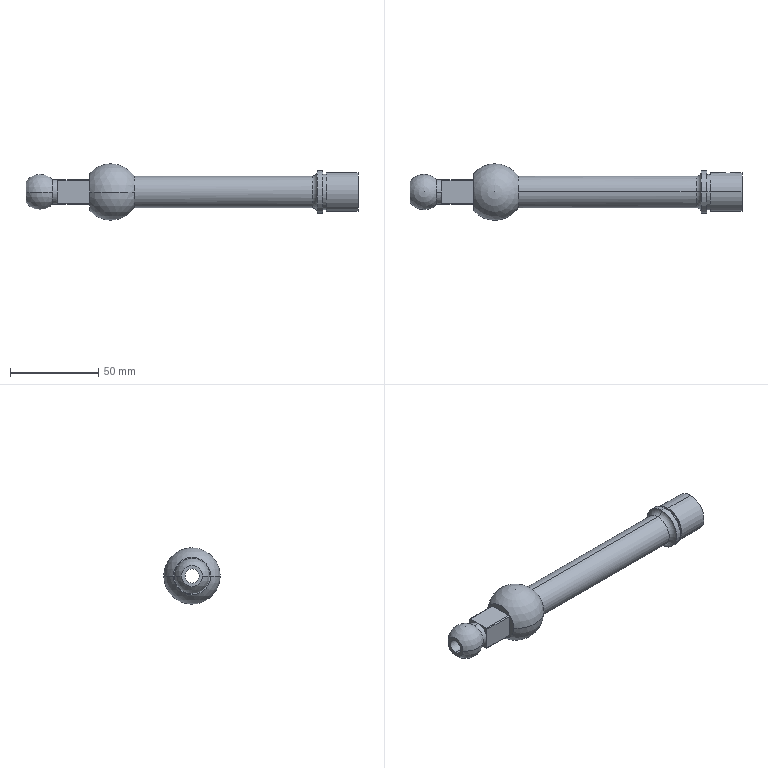Part | SolidWorks | features ICE 2, Revolution 1 | 1 solid | 42 faces | box 188 x 32 x 32 mm | volume 46322 mm3 | cylinder 20 | plane 14 | sphere 4 | torus 2 | cone 2 | commonest cylinder face diameters 19 x4 5 x2 8 x2 14 x2 17.3 x2 18 x2
STEP:
#1=CARTESIAN_POINT('',(246.379,32.914,-2.5));
#2=VERTEX_POINT('',#1);
#3=CARTESIAN_POINT('',(246.379,32.914,2.5));
#4=VERTEX_POINT('',#3);
#5=CARTESIAN_POINT('',(246.379,32.914,-2.5));
#6=CARTESIAN_POINT('',(246.214,32.914,-2.5));
#7=CARTESIAN_POINT('',(246.051,32.918,-2.484));
#8=CARTESIAN_POINT('',(245.73,32.932,-2.42));
#9=CARTESIAN_POINT('',(245.571,32.943,-2.371));
#10=CARTESIAN_POINT('',(245.269,32.97,-2.246));
#11=CARTESIAN_POINT('',(245.125,32.986,-2.169));
#12=CARTESIAN_POINT('',(244.854,33.021,-1.988));
#13=CARTESIAN_POINT('',(244.726,33.04,-1.882));
#14=CARTESIAN_POINT('',(244.381,33.096,-1.538));
#15=CARTESIAN_POINT('',(244.195,33.133,-1.259));
#16=CARTESIAN_POINT('',(244.008,33.173,-0.8084));
#17=CARTESIAN_POINT('',(243.96,33.184,-0.6503));
#18=CARTESIAN_POINT('',(243.895,33.198,-0.3273));
#19=CARTESIAN_POINT('',(243.879,33.202,-0.1647));
#20=CARTESIAN_POINT('',(243.879,33.202,0.1627));
#21=CARTESIAN_POINT('',(243.896,33.198,0.329));
#22=CARTESIAN_POINT('',(243.96,33.184,0.65));
#23=CARTESIAN_POINT('',(244.007,33.173,0.8062));
#24=CARTESIAN_POINT('',(244.196,33.133,1.261));
#25=CARTESIAN_POINT('',(244.38,33.096,1.536));
#26=CARTESIAN_POINT('',(244.728,33.04,1.884));
#27=CARTESIAN_POINT('',(244.854,33.021,1.987));
#28=CARTESIAN_POINT('',(245.124,32.986,2.168));
#29=CARTESIAN_POINT('',(245.27,32.97,2.247));
#30=CARTESIAN_POINT('',(245.572,32.943,2.372));
#31=CARTESIAN_POINT('',(245.728,32.932,2.419));
#32=CARTESIAN_POINT('',(246.05,32.918,2.484));
#33=CARTESIAN_POINT('',(246.216,32.914,2.5));
#34=CARTESIAN_POINT('',(246.379,32.914,2.5));
#35=B_SPLINE_CURVE_WITH_KNOTS('',3,(#5,#6,#7,#8,#9,#10,#11,#12,#13,#14,#15,#16,#17,#18,#19,#20,#21,#22,#23,#24,#25,#26,#27,#28,#29,#30,#31,#32,#33,#34),.UNSPECIFIED.,.F.,.F.,(4,2,2,2,2,2,2,2,2,2,2,2,2,2,4),(0.,0.0004901,0.0009802,0.00147,0.00196,0.002941,0.003431,0.003921,0.004411,0.004901,0.005881,0.006371,0.006862,0.007352,0.007842),.UNSPECIFIED.);
#36=EDGE_CURVE('',#2,#4,#35,.T.);
#37=ORIENTED_EDGE('',*,*,#36,.T.);
#38=CARTESIAN_POINT('',(246.379,30.482,2.5));
#39=VERTEX_POINT('',#38);
#40=CARTESIAN_POINT('',(246.379,39.202,2.5));
#41=DIRECTION('',(0.,-1.,0.));
#42=VECTOR('',#41,1000.);
#43=LINE('',#40,#42);
#44=EDGE_CURVE('',#4,#39,#43,.T.);
#45=ORIENTED_EDGE('',*,*,#44,.T.);
#46=CARTESIAN_POINT('',(246.379,30.482,-2.5));
#47=VERTEX_POINT('',#46);
#48=CARTESIAN_POINT('',(246.379,30.482,2.5));
#49=CARTESIAN_POINT('',(246.052,30.482,2.5));
#50=CARTESIAN_POINT('',(245.721,30.503,2.434));
#51=CARTESIAN_POINT('',(245.27,30.555,2.246));
#52=CARTESIAN_POINT('',(245.123,30.576,2.168));
#53=CARTESIAN_POINT('',(244.853,30.621,1.986));
#54=CARTESIAN_POINT('',(244.727,30.645,1.884));
#55=CARTESIAN_POINT('',(244.497,30.693,1.653));
#56=CARTESIAN_POINT('',(244.392,30.717,1.526));
#57=CARTESIAN_POINT('',(244.212,30.761,1.256));
#58=CARTESIAN_POINT('',(244.135,30.781,1.113));
#59=CARTESIAN_POINT('',(244.008,30.815,0.8077));
#60=CARTESIAN_POINT('',(243.96,30.829,0.6513));
#61=CARTESIAN_POINT('',(243.896,30.847,0.331));
#62=CARTESIAN_POINT('',(243.879,30.852,0.1651));
#63=CARTESIAN_POINT('',(243.879,30.852,-0.1645));
#64=CARTESIAN_POINT('',(243.895,30.847,-0.3273));
#65=CARTESIAN_POINT('',(243.959,30.829,-0.6493));
#66=CARTESIAN_POINT('',(244.008,30.815,-0.8088));
#67=CARTESIAN_POINT('',(244.196,30.765,-1.261));
#68=CARTESIAN_POINT('',(244.382,30.717,-1.538));
#69=CARTESIAN_POINT('',(244.726,30.645,-1.882));
#70=CARTESIAN_POINT('',(244.853,30.621,-1.987));
#71=CARTESIAN_POINT('',(245.124,30.576,-2.168));
#72=CARTESIAN_POINT('',(245.267,30.555,-2.245));
#73=CARTESIAN_POINT('',(245.569,30.521,-2.37));
#74=CARTESIAN_POINT('',(245.728,30.506,-2.419));
#75=CARTESIAN_POINT('',(246.05,30.487,-2.484));
#76=CARTESIAN_POINT('',(246.213,30.482,-2.5));
#77=CARTESIAN_POINT('',(246.379,30.482,-2.5));
#78=B_SPLINE_CURVE_WITH_KNOTS('',3,(#48,#49,#50,#51,#52,#53,#54,#55,#56,#57,#58,#59,#60,#61,#62,#63,#64,#65,#66,#67,#68,#69,#70,#71,#72,#73,#74,#75,#76,#77),.UNSPECIFIED.,.F.,.F.,(4,2,2,2,2,2,2,2,2,2,2,2,2,2,4),(0.007858,0.00884,0.009331,0.009822,0.01031,0.0108,0.0113,0.01179,0.01228,0.01277,0.01375,0.01424,0.01473,0.01522,0.01571),.UNSPECIFIED.);
#79=EDGE_CURVE('',#39,#47,#78,.T.);
#80=ORIENTED_EDGE('',*,*,#79,.T.);
#81=CARTESIAN_POINT('',(246.379,39.202,-2.5));
#82=DIRECTION('',(0.,-1.,0.));
#83=VECTOR('',#82,1000.);
#84=LINE('',#81,#83);
#85=EDGE_CURVE('',#2,#47,#84,.T.);
#86=ORIENTED_EDGE('',*,*,#85,.F.);
#87=EDGE_LOOP('',(#37,#45,#80,#86));
#88=FACE_OUTER_BOUND('',#87,.T.);
#89=CARTESIAN_POINT('',(246.379,39.202,0.));
#90=DIRECTION('',(0.,-1.,0.));
#91=DIRECTION('',(0.,0.,-1.));
#92=AXIS2_PLACEMENT_3D('',#89,#90,#91);
#93=CYLINDRICAL_SURFACE('',#92,2.5);
#94=ADVANCED_FACE('',(#88),#93,.F.);
#95=CARTESIAN_POINT('',(228.379,22.202,9.));
#96=VERTEX_POINT('',#95);
#97=CARTESIAN_POINT('',(228.379,22.202,-9.));
#98=VERTEX_POINT('',#97);
#99=CARTESIAN_POINT('',(228.379,22.202,0.));
#100=DIRECTION('',(-1.,0.,0.));
#101=DIRECTION('',(0.,0.,1.));
#102=AXIS2_PLACEMENT_3D('',#99,#100,#101);
#103=CIRCLE('',#102,9.);
#104=EDGE_CURVE('',#96,#98,#103,.T.);
#105=ORIENTED_EDGE('',*,*,#104,.T.);
#106=CARTESIAN_POINT('',(127.608,22.202,-9.));
#107=VERTEX_POINT('',#106);
#108=CARTESIAN_POINT('',(62.379,22.202,-9.));
#109=DIRECTION('',(-1.,0.,0.));
#110=VECTOR('',#109,1000.);
#111=LINE('',#108,#110);
#112=EDGE_CURVE('',#98,#107,#111,.T.);
#113=ORIENTED_EDGE('',*,*,#112,.T.);
#114=CARTESIAN_POINT('',(127.608,31.202,0.));
#115=VERTEX_POINT('',#114);
#116=CARTESIAN_POINT('',(127.608,22.202,0.));
#117=DIRECTION('',(-1.,0.,0.));
#118=DIRECTION('',(0.,0.,1.));
#119=AXIS2_PLACEMENT_3D('',#116,#117,#118);
#120=CIRCLE('',#119,9.);
#121=EDGE_CURVE('',#115,#107,#120,.T.);
#122=ORIENTED_EDGE('',*,*,#121,.F.);
#123=CARTESIAN_POINT('',(127.608,22.202,9.));
#124=VERTEX_POINT('',#123);
#125=CARTESIAN_POINT('',(127.608,22.202,0.));
#126=DIRECTION('',(-1.,0.,0.));
#127=DIRECTION('',(0.,0.,1.));
#128=AXIS2_PLACEMENT_3D('',#125,#126,#127);
#129=CIRCLE('',#128,9.);
#130=EDGE_CURVE('',#124,#115,#129,.T.);
#131=ORIENTED_EDGE('',*,*,#130,.F.);
#132=CARTESIAN_POINT('',(62.379,22.202,9.));
#133=DIRECTION('',(-1.,0.,0.));
#134=VECTOR('',#133,1000.);
#135=LINE('',#132,#134);
#136=EDGE_CURVE('',#96,#124,#135,.T.);
#137=ORIENTED_EDGE('',*,*,#136,.F.);
#138=EDGE_LOOP('',(#105,#113,#122,#131,#137));
#139=FACE_OUTER_BOUND('',#138,.T.);
#140=CARTESIAN_POINT('',(62.379,22.202,0.));
#141=DIRECTION('',(-1.,0.,0.));
#142=DIRECTION('',(0.,0.,1.));
#143=AXIS2_PLACEMENT_3D('',#140,#141,#142);
#144=CYLINDRICAL_SURFACE('',#143,9.);
#145=ADVANCED_FACE('',(#139),#144,.T.);
#146=CARTESIAN_POINT('',(228.379,22.202,0.));
#147=DIRECTION('',(-1.,0.,0.));
#148=DIRECTION('',(0.,0.,1.));
#149=AXIS2_PLACEMENT_3D('',#146,#147,#148);
#150=CIRCLE('',#149,9.);
#151=EDGE_CURVE('',#98,#96,#150,.T.);
#152=ORIENTED_EDGE('',*,*,#151,.F.);
#153=CARTESIAN_POINT('',(231.379,22.202,-12.));
#154=VERTEX_POINT('',#153);
#155=CARTESIAN_POINT('',(228.379,22.202,-12.));
#156=DIRECTION('',(0.,1.,0.));
#157=DIRECTION('',(0.,0.,1.));
#158=AXIS2_PLACEMENT_3D('',#155,#156,#157);
#159=CIRCLE('',#158,3.);
#160=EDGE_CURVE('',#98,#154,#159,.T.);
#161=ORIENTED_EDGE('',*,*,#160,.T.);
#162=CARTESIAN_POINT('',(231.379,22.202,12.));
#163=VERTEX_POINT('',#162);
#164=CARTESIAN_POINT('',(231.379,22.202,0.));
#165=DIRECTION('',(-1.,0.,0.));
#166=DIRECTION('',(0.,0.,1.));
#167=AXIS2_PLACEMENT_3D('',#164,#165,#166);
#168=CIRCLE('',#167,12.);
#169=EDGE_CURVE('',#154,#163,#168,.T.);
#170=ORIENTED_EDGE('',*,*,#169,.T.);
#171=CARTESIAN_POINT('',(228.379,22.202,12.));
#172=DIRECTION('',(0.,-1.,0.));
#173=DIRECTION('',(0.,0.,-1.));
#174=AXIS2_PLACEMENT_3D('',#171,#172,#173);
#175=CIRCLE('',#174,3.);
#176=EDGE_CURVE('',#96,#163,#175,.T.);
#177=ORIENTED_EDGE('',*,*,#176,.F.);
#178=EDGE_LOOP('',(#152,#161,#170,#177));
#179=FACE_OUTER_BOUND('',#178,.T.);
#180=CARTESIAN_POINT('',(228.379,22.202,0.));
#181=DIRECTION('',(-1.,0.,0.));
#182=DIRECTION('',(0.,0.,1.));
#183=AXIS2_PLACEMENT_3D('',#180,#181,#182);
#184=TOROIDAL_SURFACE('',#183,12.,3.);
#185=ADVANCED_FACE('',(#179),#184,.F.);
#186=CARTESIAN_POINT('',(234.379,22.202,12.));
#187=VERTEX_POINT('',#186);
#188=CARTESIAN_POINT('',(234.379,22.202,-12.));
#189=VERTEX_POINT('',#188);
#190=CARTESIAN_POINT('',(234.379,22.202,0.));
#191=DIRECTION('',(-1.,0.,0.));
#192=DIRECTION('',(0.,0.,1.));
#193=AXIS2_PLACEMENT_3D('',#190,#191,#192);
#194=CIRCLE('',#193,12.);
#195=EDGE_CURVE('',#187,#189,#194,.T.);
#196=ORIENTED_EDGE('',*,*,#195,.T.);
#197=CARTESIAN_POINT('',(62.379,22.202,-12.));
#198=DIRECTION('',(-1.,0.,0.));
#199=VECTOR('',#198,1000.);
#200=LINE('',#197,#199);
#201=EDGE_CURVE('',#189,#154,#200,.T.);
#202=ORIENTED_EDGE('',*,*,#201,.T.);
#203=CARTESIAN_POINT('',(231.379,22.202,0.));
#204=DIRECTION('',(-1.,0.,0.));
#205=DIRECTION('',(0.,0.,1.));
#206=AXIS2_PLACEMENT_3D('',#203,#204,#205);
#207=CIRCLE('',#206,12.);
#208=EDGE_CURVE('',#163,#154,#207,.T.);
#209=ORIENTED_EDGE('',*,*,#208,.F.);
#210=CARTESIAN_POINT('',(62.379,22.202,12.));
#211=DIRECTION('',(-1.,0.,0.));
#212=VECTOR('',#211,1000.);
#213=LINE('',#210,#212);
#214=EDGE_CURVE('',#187,#163,#213,.T.);
#215=ORIENTED_EDGE('',*,*,#214,.F.);
#216=EDGE_LOOP('',(#196,#202,#209,#215));
#217=FACE_OUTER_BOUND('',#216,.T.);
#218=CARTESIAN_POINT('',(62.379,22.202,0.));
#219=DIRECTION('',(-1.,0.,0.));
#220=DIRECTION('',(0.,0.,1.));
#221=AXIS2_PLACEMENT_3D('',#218,#219,#220);
#222=CYLINDRICAL_SURFACE('',#221,12.);
#223=ADVANCED_FACE('',(#217),#222,.T.);
#224=CARTESIAN_POINT('',(236.379,22.202,10.));
#225=VERTEX_POINT('',#224);
#226=CARTESIAN_POINT('',(236.379,22.202,-10.));
#227=VERTEX_POINT('',#226);
#228=CARTESIAN_POINT('',(236.379,22.202,0.));
#229=DIRECTION('',(-1.,0.,0.));
#230=DIRECTION('',(0.,0.,1.));
#231=AXIS2_PLACEMENT_3D('',#228,#229,#230);
#232=CIRCLE('',#231,10.);
#233=EDGE_CURVE('',#225,#227,#232,.T.);
#234=ORIENTED_EDGE('',*,*,#233,.T.);
#235=CARTESIAN_POINT('',(234.379,22.202,-10.));
#236=VERTEX_POINT('',#235);
#237=CARTESIAN_POINT('',(62.379,22.202,-10.));
#238=DIRECTION('',(-1.,0.,0.));
#239=VECTOR('',#238,1000.);
#240=LINE('',#237,#239);
#241=EDGE_CURVE('',#227,#236,#240,.T.);
#242=ORIENTED_EDGE('',*,*,#241,.T.);
#243=CARTESIAN_POINT('',(234.379,22.202,10.));
#244=VERTEX_POINT('',#243);
#245=CARTESIAN_POINT('',(234.379,22.202,0.));
#246=DIRECTION('',(-1.,0.,0.));
#247=DIRECTION('',(0.,0.,1.));
#248=AXIS2_PLACEMENT_3D('',#245,#246,#247);
#249=CIRCLE('',#248,10.);
#250=EDGE_CURVE('',#244,#236,#249,.T.);
#251=ORIENTED_EDGE('',*,*,#250,.F.);
#252=CARTESIAN_POINT('',(62.379,22.202,10.));
#253=DIRECTION('',(-1.,0.,0.));
#254=VECTOR('',#253,1000.);
#255=LINE('',#252,#254);
#256=EDGE_CURVE('',#225,#244,#255,.T.);
#257=ORIENTED_EDGE('',*,*,#256,.F.);
#258=EDGE_LOOP('',(#234,#242,#251,#257));
#259=FACE_OUTER_BOUND('',#258,.T.);
#260=CARTESIAN_POINT('',(62.379,22.202,0.));
#261=DIRECTION('',(-1.,0.,0.));
#262=DIRECTION('',(0.,0.,1.));
#263=AXIS2_PLACEMENT_3D('',#260,#261,#262);
#264=CYLINDRICAL_SURFACE('',#263,10.);
#265=ADVANCED_FACE('',(#259),#264,.T.);
#266=CARTESIAN_POINT('',(234.379,22.202,-4.));
#267=VERTEX_POINT('',#266);
#268=CARTESIAN_POINT('',(234.379,22.202,4.));
#269=VERTEX_POINT('',#268);
#270=CARTESIAN_POINT('',(234.379,22.202,0.));
#271=DIRECTION('',(-1.,0.,0.));
#272=DIRECTION('',(0.,0.,1.));
#273=AXIS2_PLACEMENT_3D('',#270,#271,#272);
#274=CIRCLE('',#273,4.);
#275=EDGE_CURVE('',#267,#269,#274,.T.);
#276=ORIENTED_EDGE('',*,*,#275,.T.);
#277=CARTESIAN_POINT('',(237.379,22.202,8.65));
#278=VERTEX_POINT('',#277);
#279=CARTESIAN_POINT('',(234.379,22.202,4.));
#280=DIRECTION('',(0.5421,0.,0.8403));
#281=VECTOR('',#280,1000.);
#282=LINE('',#279,#281);
#283=EDGE_CURVE('',#269,#278,#282,.T.);
#284=ORIENTED_EDGE('',*,*,#283,.T.);
#285=CARTESIAN_POINT('',(237.379,22.202,-8.65));
#286=VERTEX_POINT('',#285);
#287=CARTESIAN_POINT('',(237.379,22.202,0.));
#288=DIRECTION('',(-1.,0.,0.));
#289=DIRECTION('',(0.,0.,1.));
#290=AXIS2_PLACEMENT_3D('',#287,#288,#289);
#291=CIRCLE('',#290,8.65);
#292=EDGE_CURVE('',#286,#278,#291,.T.);
#293=ORIENTED_EDGE('',*,*,#292,.F.);
#294=CARTESIAN_POINT('',(234.379,22.202,-4.));
#295=DIRECTION('',(0.5421,0.,-0.8403));
#296=VECTOR('',#295,1000.);
#297=LINE('',#294,#296);
#298=EDGE_CURVE('',#267,#286,#297,.T.);
#299=ORIENTED_EDGE('',*,*,#298,.F.);
#300=EDGE_LOOP('',(#276,#284,#293,#299));
#301=FACE_OUTER_BOUND('',#300,.T.);
#302=CARTESIAN_POINT('',(234.379,22.202,0.));
#303=DIRECTION('',(1.,0.,0.));
#304=DIRECTION('',(0.,0.,-1.));
#305=AXIS2_PLACEMENT_3D('',#302,#303,#304);
#306=CONICAL_SURFACE('',#305,4.,0.9978);
#307=ADVANCED_FACE('',(#301),#306,.F.);
#308=ORIENTED_EDGE('',*,*,#275,.F.);
#309=CARTESIAN_POINT('',(66.379,22.202,-4.));
#310=VERTEX_POINT('',#309);
#311=CARTESIAN_POINT('',(62.379,22.202,-4.));
#312=DIRECTION('',(-1.,0.,0.));
#313=VECTOR('',#312,1000.);
#314=LINE('',#311,#313);
#315=EDGE_CURVE('',#267,#310,#314,.T.);
#316=ORIENTED_EDGE('',*,*,#315,.T.);
#317=CARTESIAN_POINT('',(66.379,22.202,4.));
#318=VERTEX_POINT('',#317);
#319=CARTESIAN_POINT('',(66.379,22.202,0.));
#320=DIRECTION('',(-1.,0.,0.));
#321=DIRECTION('',(0.,0.,1.));
#322=AXIS2_PLACEMENT_3D('',#319,#320,#321);
#323=CIRCLE('',#322,4.);
#324=EDGE_CURVE('',#310,#318,#323,.T.);
#325=ORIENTED_EDGE('',*,*,#324,.T.);
#326=CARTESIAN_POINT('',(62.379,22.202,4.));
#327=DIRECTION('',(-1.,0.,0.));
#328=VECTOR('',#327,1000.);
#329=LINE('',#326,#328);
#330=EDGE_CURVE('',#269,#318,#329,.T.);
#331=ORIENTED_EDGE('',*,*,#330,.F.);
#332=EDGE_LOOP('',(#308,#316,#325,#331));
#333=FACE_OUTER_BOUND('',#332,.T.);
#334=CARTESIAN_POINT('',(62.379,22.202,0.));
#335=DIRECTION('',(-1.,0.,0.));
#336=DIRECTION('',(0.,0.,1.));
#337=AXIS2_PLACEMENT_3D('',#334,#335,#336);
#338=CYLINDRICAL_SURFACE('',#337,4.);
#339=ADVANCED_FACE('',(#333),#338,.F.);
#340=CARTESIAN_POINT('',(81.379,29.343,0.));
#341=VERTEX_POINT('',#340);
#342=CARTESIAN_POINT('',(81.379,15.06,0.));
#343=VERTEX_POINT('',#342);
#344=CARTESIAN_POINT('',(81.379,22.202,0.));
#345=DIRECTION('',(-1.,0.,0.));
#346=DIRECTION('',(0.,0.,1.));
#347=AXIS2_PLACEMENT_3D('',#344,#345,#346);
#348=CIRCLE('',#347,7.141);
#349=EDGE_CURVE('',#341,#343,#348,.T.);
#350=ORIENTED_EDGE('',*,*,#349,.T.);
#351=CARTESIAN_POINT('',(66.379,16.202,0.));
#352=VERTEX_POINT('',#351);
#353=CARTESIAN_POINT('',(74.379,22.202,0.));
#354=DIRECTION('',(0.,0.,-1.));
#355=DIRECTION('',(0.,1.,0.));
#356=AXIS2_PLACEMENT_3D('',#353,#354,#355);
#357=CIRCLE('',#356,10.);
#358=EDGE_CURVE('',#343,#352,#357,.T.);
#359=ORIENTED_EDGE('',*,*,#358,.T.);
#360=CARTESIAN_POINT('',(66.379,28.202,0.));
#361=VERTEX_POINT('',#360);
#362=CARTESIAN_POINT('',(66.379,22.202,0.));
#363=DIRECTION('',(-1.,0.,0.));
#364=DIRECTION('',(0.,0.,1.));
#365=AXIS2_PLACEMENT_3D('',#362,#363,#364);
#366=CIRCLE('',#365,6.);
#367=EDGE_CURVE('',#361,#352,#366,.T.);
#368=ORIENTED_EDGE('',*,*,#367,.F.);
#369=CARTESIAN_POINT('',(74.379,22.202,0.));
#370=DIRECTION('',(0.,0.,1.));
#371=DIRECTION('',(1.,0.,0.));
#372=AXIS2_PLACEMENT_3D('',#369,#370,#371);
#373=CIRCLE('',#372,10.);
#374=EDGE_CURVE('',#341,#361,#373,.T.);
#375=ORIENTED_EDGE('',*,*,#374,.F.);
#376=EDGE_LOOP('',(#350,#359,#368,#375));
#377=FACE_OUTER_BOUND('',#376,.T.);
#378=CARTESIAN_POINT('',(74.379,22.202,0.));
#379=DIRECTION('',(0.,0.,-1.));
#380=DIRECTION('',(0.,1.,0.));
#381=AXIS2_PLACEMENT_3D('',#378,#379,#380);
#382=SPHERICAL_SURFACE('',#381,10.);
#383=ADVANCED_FACE('',(#377),#382,.T.);
#384=CARTESIAN_POINT('',(84.379,29.202,0.));
#385=VERTEX_POINT('',#384);
#386=CARTESIAN_POINT('',(84.379,22.202,-7.));
#387=VERTEX_POINT('',#386);
#388=CARTESIAN_POINT('',(84.379,22.202,0.));
#389=DIRECTION('',(-1.,0.,0.));
#390=DIRECTION('',(0.,0.,1.));
#391=AXIS2_PLACEMENT_3D('',#388,#389,#390);
#392=CIRCLE('',#391,7.);
#393=EDGE_CURVE('',#385,#387,#392,.T.);
#394=ORIENTED_EDGE('',*,*,#393,.T.);
#395=CARTESIAN_POINT('',(81.379,22.202,-7.));
#396=VERTEX_POINT('',#395);
#397=CARTESIAN_POINT('',(62.379,22.202,-7.));
#398=DIRECTION('',(-1.,0.,0.));
#399=VECTOR('',#398,1000.);
#400=LINE('',#397,#399);
#401=EDGE_CURVE('',#387,#396,#400,.T.);
#402=ORIENTED_EDGE('',*,*,#401,.T.);
#403=CARTESIAN_POINT('',(81.379,22.202,7.));
#404=VERTEX_POINT('',#403);
#405=CARTESIAN_POINT('',(81.379,22.202,0.));
#406=DIRECTION('',(-1.,0.,0.));
#407=DIRECTION('',(0.,0.,1.));
#408=AXIS2_PLACEMENT_3D('',#405,#406,#407);
#409=CIRCLE('',#408,7.);
#410=EDGE_CURVE('',#404,#396,#409,.T.);
#411=ORIENTED_EDGE('',*,*,#410,.F.);
#412=CARTESIAN_POINT('',(84.379,22.202,7.));
#413=VERTEX_POINT('',#412);
#414=CARTESIAN_POINT('',(62.379,22.202,7.));
#415=DIRECTION('',(-1.,0.,0.));
#416=VECTOR('',#415,1000.);
#417=LINE('',#414,#416);
#418=EDGE_CURVE('',#413,#404,#417,.T.);
#419=ORIENTED_EDGE('',*,*,#418,.F.);
#420=CARTESIAN_POINT('',(84.379,22.202,0.));
#421=DIRECTION('',(-1.,0.,0.));
#422=DIRECTION('',(0.,0.,1.));
#423=AXIS2_PLACEMENT_3D('',#420,#421,#422);
#424=CIRCLE('',#423,7.);
#425=EDGE_CURVE('',#413,#385,#424,.T.);
#426=ORIENTED_EDGE('',*,*,#425,.T.);
#427=EDGE_LOOP('',(#394,#402,#411,#419,#426));
#428=FACE_OUTER_BOUND('',#427,.T.);
#429=CARTESIAN_POINT('',(62.379,22.202,0.));
#430=DIRECTION('',(-1.,0.,0.));
#431=DIRECTION('',(0.,0.,1.));
#432=AXIS2_PLACEMENT_3D('',#429,#430,#431);
#433=CYLINDRICAL_SURFACE('',#432,7.);
#434=ADVANCED_FACE('',(#428),#433,.T.);
#435=ORIENTED_EDGE('',*,*,#121,.T.);
#436=CARTESIAN_POINT('',(127.608,13.202,0.));
#437=VERTEX_POINT('',#436);
#438=CARTESIAN_POINT('',(127.608,22.202,0.));
#439=DIRECTION('',(-1.,0.,0.));
#440=DIRECTION('',(0.,0.,1.));
#441=AXIS2_PLACEMENT_3D('',#438,#439,#440);
#442=CIRCLE('',#441,9.);
#443=EDGE_CURVE('',#107,#437,#442,.T.);
#444=ORIENTED_EDGE('',*,*,#443,.T.);
#445=CARTESIAN_POINT('',(102.379,11.619,0.));
#446=VERTEX_POINT('',#445);
#447=CARTESIAN_POINT('',(114.379,22.202,0.));
#448=DIRECTION('',(0.,0.,-1.));
#449=DIRECTION('',(0.,1.,0.));
#450=AXIS2_PLACEMENT_3D('',#447,#448,#449);
#451=CIRCLE('',#450,16.);
#452=EDGE_CURVE('',#437,#446,#451,.T.);
#453=ORIENTED_EDGE('',*,*,#452,.T.);
#454=CARTESIAN_POINT('',(102.379,32.785,0.));
#455=VERTEX_POINT('',#454);
#456=CARTESIAN_POINT('',(102.379,22.202,0.));
#457=DIRECTION('',(-1.,0.,0.));
#458=DIRECTION('',(0.,0.,1.));
#459=AXIS2_PLACEMENT_3D('',#456,#457,#458);
#460=CIRCLE('',#459,10.583);
#461=EDGE_CURVE('',#455,#446,#460,.T.);
#462=ORIENTED_EDGE('',*,*,#461,.F.);
#463=CARTESIAN_POINT('',(114.379,22.202,0.));
#464=DIRECTION('',(0.,0.,1.));
#465=DIRECTION('',(1.,0.,0.));
#466=AXIS2_PLACEMENT_3D('',#463,#464,#465);
#467=CIRCLE('',#466,16.);
#468=EDGE_CURVE('',#115,#455,#467,.T.);
#469=ORIENTED_EDGE('',*,*,#468,.F.);
#470=EDGE_LOOP('',(#435,#444,#453,#462,#469));
#471=FACE_OUTER_BOUND('',#470,.T.);
#472=CARTESIAN_POINT('',(114.379,22.202,0.));
#473=DIRECTION('',(0.,0.,-1.));
#474=DIRECTION('',(0.,1.,0.));
#475=AXIS2_PLACEMENT_3D('',#472,#473,#474);
#476=SPHERICAL_SURFACE('',#475,16.);
#477=ADVANCED_FACE('',(#471),#476,.T.);
#478=ORIENTED_EDGE('',*,*,#36,.F.);
#479=CARTESIAN_POINT('',(246.379,32.914,2.5));
#480=CARTESIAN_POINT('',(246.706,32.914,2.5));
#481=CARTESIAN_POINT('',(247.036,32.93,2.434));
#482=CARTESIAN_POINT('',(247.488,32.97,2.247));
#483=CARTESIAN_POINT('',(247.634,32.986,2.169));
#484=CARTESIAN_POINT('',(247.905,33.021,1.987));
#485=CARTESIAN_POINT('',(248.031,33.04,1.884));
#486=CARTESIAN_POINT('',(248.261,33.077,1.654));
#487=CARTESIAN_POINT('',(248.367,33.096,1.525));
#488=CARTESIAN_POINT('',(248.547,33.131,1.255));
#489=CARTESIAN_POINT('',(248.624,33.146,1.112));
#490=CARTESIAN_POINT('',(248.814,33.186,0.6562));
#491=CARTESIAN_POINT('',(248.879,33.202,0.3309));
#492=CARTESIAN_POINT('',(248.879,33.202,-0.164));
#493=CARTESIAN_POINT('',(248.863,33.198,-0.3266));
#494=CARTESIAN_POINT('',(248.8,33.184,-0.6474));
#495=CARTESIAN_POINT('',(248.751,33.173,-0.8069));
#496=CARTESIAN_POINT('',(248.626,33.147,-1.109));
#497=CARTESIAN_POINT('',(248.549,33.131,-1.252));
#498=CARTESIAN_POINT('',(248.367,33.096,-1.525));
#499=CARTESIAN_POINT('',(248.263,33.077,-1.652));
#500=CARTESIAN_POINT('',(247.919,33.021,-1.996));
#501=CARTESIAN_POINT('',(247.641,32.984,-2.183));
#502=CARTESIAN_POINT('',(247.19,32.943,-2.371));
#503=CARTESIAN_POINT('',(247.031,32.932,-2.419));
#504=CARTESIAN_POINT('',(246.708,32.918,-2.484));
#505=CARTESIAN_POINT('',(246.545,32.914,-2.5));
#506=CARTESIAN_POINT('',(246.379,32.914,-2.5));
#507=B_SPLINE_CURVE_WITH_KNOTS('',3,(#479,#480,#481,#482,#483,#484,#485,#486,#487,#488,#489,#490,#491,#492,#493,#494,#495,#496,#497,#498,#499,#500,#501,#502,#503,#504,#505,#506),.UNSPECIFIED.,.F.,.F.,(4,2,2,2,2,2,2,2,2,2,2,2,2,4),(0.007842,0.008822,0.009312,0.009802,0.01029,0.01078,0.01176,0.01225,0.01274,0.01323,0.01372,0.0147,0.01519,0.01568),.UNSPECIFIED.);
#508=EDGE_CURVE('',#4,#2,#507,.T.);
#509=ORIENTED_EDGE('',*,*,#508,.F.);
#510=EDGE_LOOP('',(#478,#509));
#511=FACE_BOUND('',#510,.T.);
#512=CARTESIAN_POINT('',(254.379,22.202,11.));
#513=VERTEX_POINT('',#512);
#514=CARTESIAN_POINT('',(254.379,22.202,-11.));
#515=VERTEX_POINT('',#514);
#516=CARTESIAN_POINT('',(254.379,22.202,0.));
#517=DIRECTION('',(-1.,0.,0.));
#518=DIRECTION('',(0.,0.,1.));
#519=AXIS2_PLACEMENT_3D('',#516,#517,#518);
#520=CIRCLE('',#519,11.);
#521=EDGE_CURVE('',#513,#515,#520,.T.);
#522=ORIENTED_EDGE('',*,*,#521,.T.);
#523=CARTESIAN_POINT('',(236.379,22.202,-11.));
#524=VERTEX_POINT('',#523);
#525=CARTESIAN_POINT('',(62.379,22.202,-11.));
#526=DIRECTION('',(-1.,0.,0.));
#527=VECTOR('',#526,1000.);
#528=LINE('',#525,#527);
#529=EDGE_CURVE('',#515,#524,#528,.T.);
#530=ORIENTED_EDGE('',*,*,#529,.T.);
#531=CARTESIAN_POINT('',(236.379,22.202,11.));
#532=VERTEX_POINT('',#531);
#533=CARTESIAN_POINT('',(236.379,22.202,0.));
#534=DIRECTION('',(-1.,0.,0.));
#535=DIRECTION('',(0.,0.,1.));
#536=AXIS2_PLACEMENT_3D('',#533,#534,#535);
#537=CIRCLE('',#536,11.);
#538=EDGE_CURVE('',#532,#524,#537,.T.);
#539=ORIENTED_EDGE('',*,*,#538,.F.);
#540=CARTESIAN_POINT('',(62.379,22.202,11.));
#541=DIRECTION('',(-1.,0.,0.));
#542=VECTOR('',#541,1000.);
#543=LINE('',#540,#542);
#544=EDGE_CURVE('',#513,#532,#543,.T.);
#545=ORIENTED_EDGE('',*,*,#544,.F.);
#546=EDGE_LOOP('',(#522,#530,#539,#545));
#547=FACE_OUTER_BOUND('',#546,.T.);
#548=CARTESIAN_POINT('',(62.379,22.202,0.));
#549=DIRECTION('',(-1.,0.,0.));
#550=DIRECTION('',(0.,0.,1.));
#551=AXIS2_PLACEMENT_3D('',#548,#549,#550);
#552=CYLINDRICAL_SURFACE('',#551,11.);
#553=ADVANCED_FACE('',(#511,#547),#552,.T.);
#554=CARTESIAN_POINT('',(254.379,22.202,-8.65));
#555=VERTEX_POINT('',#554);
#556=CARTESIAN_POINT('',(254.379,22.202,8.65));
#557=VERTEX_POINT('',#556);
#558=CARTESIAN_POINT('',(254.379,22.202,0.));
#559=DIRECTION('',(-1.,0.,0.));
#560=DIRECTION('',(0.,0.,1.));
#561=AXIS2_PLACEMENT_3D('',#558,#559,#560);
#562=CIRCLE('',#561,8.65);
#563=EDGE_CURVE('',#555,#557,#562,.T.);
#564=ORIENTED_EDGE('',*,*,#563,.F.);
#565=CARTESIAN_POINT('',(62.379,22.202,-8.65));
#566=DIRECTION('',(-1.,0.,0.));
#567=VECTOR('',#566,1000.);
#568=LINE('',#565,#567);
#569=EDGE_CURVE('',#555,#286,#568,.T.);
#570=ORIENTED_EDGE('',*,*,#569,.T.);
#571=ORIENTED_EDGE('',*,*,#292,.T.);
#572=CARTESIAN_POINT('',(62.379,22.202,8.65));
#573=DIRECTION('',(-1.,0.,0.));
#574=VECTOR('',#573,1000.);
#575=LINE('',#572,#574);
#576=EDGE_CURVE('',#557,#278,#575,.T.);
#577=ORIENTED_EDGE('',*,*,#576,.F.);
#578=EDGE_LOOP('',(#564,#570,#571,#577));
#579=FACE_OUTER_BOUND('',#578,.T.);
#580=CARTESIAN_POINT('',(62.379,22.202,0.));
#581=DIRECTION('',(-1.,0.,0.));
#582=DIRECTION('',(0.,0.,1.));
#583=AXIS2_PLACEMENT_3D('',#580,#581,#582);
#584=CYLINDRICAL_SURFACE('',#583,8.65);
#585=ADVANCED_FACE('',(#579),#584,.F.);
#586=ORIENTED_EDGE('',*,*,#569,.F.);
#587=CARTESIAN_POINT('',(254.379,22.202,0.));
#588=DIRECTION('',(-1.,0.,0.));
#589=DIRECTION('',(0.,0.,1.));
#590=AXIS2_PLACEMENT_3D('',#587,#588,#589);
#591=CIRCLE('',#590,8.65);
#592=EDGE_CURVE('',#557,#555,#591,.T.);
#593=ORIENTED_EDGE('',*,*,#592,.F.);
#594=ORIENTED_EDGE('',*,*,#576,.T.);
#595=CARTESIAN_POINT('',(237.379,22.202,0.));
#596=DIRECTION('',(-1.,0.,0.));
#597=DIRECTION('',(0.,0.,1.));
#598=AXIS2_PLACEMENT_3D('',#595,#596,#597);
#599=CIRCLE('',#598,8.65);
#600=EDGE_CURVE('',#278,#286,#599,.T.);
#601=ORIENTED_EDGE('',*,*,#600,.T.);
#602=EDGE_LOOP('',(#586,#593,#594,#601));
#603=FACE_OUTER_BOUND('',#602,.T.);
#604=CARTESIAN_POINT('',(246.379,30.482,-2.5));
#605=CARTESIAN_POINT('',(246.545,30.482,-2.5));
#606=CARTESIAN_POINT('',(246.709,30.487,-2.484));
#607=CARTESIAN_POINT('',(247.029,30.506,-2.42));
#608=CARTESIAN_POINT('',(247.189,30.521,-2.371));
#609=CARTESIAN_POINT('',(247.491,30.555,-2.245));
#610=CARTESIAN_POINT('',(247.634,30.576,-2.168));
#611=CARTESIAN_POINT('',(247.905,30.621,-1.987));
#612=CARTESIAN_POINT('',(248.033,30.645,-1.882));
#613=CARTESIAN_POINT('',(248.377,30.717,-1.538));
#614=CARTESIAN_POINT('',(248.563,30.765,-1.261));
#615=CARTESIAN_POINT('',(248.75,30.815,-0.8097));
#616=CARTESIAN_POINT('',(248.799,30.829,-0.6512));
#617=CARTESIAN_POINT('',(248.863,30.847,-0.328));
#618=CARTESIAN_POINT('',(248.879,30.852,-0.1651));
#619=CARTESIAN_POINT('',(248.879,30.852,0.163));
#620=CARTESIAN_POINT('',(248.863,30.847,0.3297));
#621=CARTESIAN_POINT('',(248.799,30.829,0.6511));
#622=CARTESIAN_POINT('',(248.751,30.815,0.8074));
#623=CARTESIAN_POINT('',(248.562,30.764,1.263));
#624=CARTESIAN_POINT('',(248.377,30.717,1.538));
#625=CARTESIAN_POINT('',(248.031,30.645,1.884));
#626=CARTESIAN_POINT('',(247.905,30.621,1.987));
#627=CARTESIAN_POINT('',(247.635,30.576,2.168));
#628=CARTESIAN_POINT('',(247.489,30.555,2.246));
#629=CARTESIAN_POINT('',(247.187,30.52,2.371));
#630=CARTESIAN_POINT('',(247.032,30.507,2.419));
#631=CARTESIAN_POINT('',(246.709,30.487,2.484));
#632=CARTESIAN_POINT('',(246.543,30.482,2.5));
#633=CARTESIAN_POINT('',(246.379,30.482,2.5));
#634=B_SPLINE_CURVE_WITH_KNOTS('',3,(#604,#605,#606,#607,#608,#609,#610,#611,#612,#613,#614,#615,#616,#617,#618,#619,#620,#621,#622,#623,#624,#625,#626,#627,#628,#629,#630,#631,#632,#633),.UNSPECIFIED.,.F.,.F.,(4,2,2,2,2,2,2,2,2,2,2,2,2,2,4),(0.,0.0004911,0.0009823,0.001473,0.001965,0.002947,0.003438,0.003929,0.00442,0.004911,0.005894,0.006385,0.006876,0.007367,0.007858),.UNSPECIFIED.);
#635=EDGE_CURVE('',#47,#39,#634,.T.);
#636=ORIENTED_EDGE('',*,*,#635,.F.);
#637=ORIENTED_EDGE('',*,*,#79,.F.);
#638=EDGE_LOOP('',(#636,#637));
#639=FACE_BOUND('',#638,.T.);
#640=CARTESIAN_POINT('',(62.379,22.202,0.));
#641=DIRECTION('',(-1.,0.,0.));
#642=DIRECTION('',(0.,0.,1.));
#643=AXIS2_PLACEMENT_3D('',#640,#641,#642);
#644=CYLINDRICAL_SURFACE('',#643,8.65);
#645=ADVANCED_FACE('',(#603,#639),#644,.F.);
#646=ORIENTED_EDGE('',*,*,#529,.F.);
#647=CARTESIAN_POINT('',(254.379,22.202,0.));
#648=DIRECTION('',(-1.,0.,0.));
#649=DIRECTION('',(0.,0.,1.));
#650=AXIS2_PLACEMENT_3D('',#647,#648,#649);
#651=CIRCLE('',#650,11.);
#652=EDGE_CURVE('',#515,#513,#651,.T.);
#653=ORIENTED_EDGE('',*,*,#652,.T.);
#654=ORIENTED_EDGE('',*,*,#544,.T.);
#655=CARTESIAN_POINT('',(236.379,22.202,0.));
#656=DIRECTION('',(-1.,0.,0.));
#657=DIRECTION('',(0.,0.,1.));
#658=AXIS2_PLACEMENT_3D('',#655,#656,#657);
#659=CIRCLE('',#658,11.);
#660=EDGE_CURVE('',#524,#532,#659,.T.);
#661=ORIENTED_EDGE('',*,*,#660,.F.);
#662=EDGE_LOOP('',(#646,#653,#654,#661));
#663=FACE_OUTER_BOUND('',#662,.T.);
#664=CARTESIAN_POINT('',(62.379,22.202,0.));
#665=DIRECTION('',(-1.,0.,0.));
#666=DIRECTION('',(0.,0.,1.));
#667=AXIS2_PLACEMENT_3D('',#664,#665,#666);
#668=CYLINDRICAL_SURFACE('',#667,11.);
#669=ADVANCED_FACE('',(#663),#668,.T.);
#670=CARTESIAN_POINT('',(102.379,28.624,7.));
#671=VERTEX_POINT('',#670);
#672=CARTESIAN_POINT('',(84.379,28.624,7.));
#673=VERTEX_POINT('',#672);
#674=CARTESIAN_POINT('',(62.379,28.624,7.));
#675=DIRECTION('',(-1.,0.,0.));
#676=VECTOR('',#675,1000.);
#677=LINE('',#674,#676);
#678=EDGE_CURVE('',#671,#673,#677,.T.);
#679=ORIENTED_EDGE('',*,*,#678,.F.);
#680=CARTESIAN_POINT('',(102.379,29.202,6.423));
#681=VERTEX_POINT('',#680);
#682=CARTESIAN_POINT('',(102.379,22.202,0.));
#683=DIRECTION('',(-1.,0.,0.));
#684=DIRECTION('',(0.,0.,1.));
#685=AXIS2_PLACEMENT_3D('',#682,#683,#684);
#686=CIRCLE('',#685,9.5);
#687=EDGE_CURVE('',#671,#681,#686,.T.);
#688=ORIENTED_EDGE('',*,*,#687,.T.);
#689=CARTESIAN_POINT('',(84.379,29.202,6.423));
#690=VERTEX_POINT('',#689);
#691=CARTESIAN_POINT('',(62.379,29.202,6.423));
#692=DIRECTION('',(1.,0.,0.));
#693=VECTOR('',#692,1000.);
#694=LINE('',#691,#693);
#695=EDGE_CURVE('',#690,#681,#694,.T.);
#696=ORIENTED_EDGE('',*,*,#695,.F.);
#697=CARTESIAN_POINT('',(84.379,22.202,0.));
#698=DIRECTION('',(-1.,0.,0.));
#699=DIRECTION('',(0.,0.,1.));
#700=AXIS2_PLACEMENT_3D('',#697,#698,#699);
#701=CIRCLE('',#700,9.5);
#702=EDGE_CURVE('',#673,#690,#701,.T.);
#703=ORIENTED_EDGE('',*,*,#702,.F.);
#704=EDGE_LOOP('',(#679,#688,#696,#703));
#705=FACE_OUTER_BOUND('',#704,.T.);
#706=CARTESIAN_POINT('',(62.379,22.202,0.));
#707=DIRECTION('',(-1.,0.,0.));
#708=DIRECTION('',(0.,0.,1.));
#709=AXIS2_PLACEMENT_3D('',#706,#707,#708);
#710=CYLINDRICAL_SURFACE('',#709,9.5);
#711=ADVANCED_FACE('',(#705),#710,.T.);
#712=CARTESIAN_POINT('',(84.379,15.779,7.));
#713=VERTEX_POINT('',#712);
#714=CARTESIAN_POINT('',(102.379,15.779,7.));
#715=VERTEX_POINT('',#714);
#716=CARTESIAN_POINT('',(62.379,15.779,7.));
#717=DIRECTION('',(1.,0.,0.));
#718=VECTOR('',#717,1000.);
#719=LINE('',#716,#718);
#720=EDGE_CURVE('',#713,#715,#719,.T.);
#721=ORIENTED_EDGE('',*,*,#720,.F.);
#722=CARTESIAN_POINT('',(84.379,15.202,6.423));
#723=VERTEX_POINT('',#722);
#724=CARTESIAN_POINT('',(84.379,22.202,0.));
#725=DIRECTION('',(-1.,0.,0.));
#726=DIRECTION('',(0.,0.,1.));
#727=AXIS2_PLACEMENT_3D('',#724,#725,#726);
#728=CIRCLE('',#727,9.5);
#729=EDGE_CURVE('',#723,#713,#728,.T.);
#730=ORIENTED_EDGE('',*,*,#729,.F.);
#731=CARTESIAN_POINT('',(102.379,15.202,6.423));
#732=VERTEX_POINT('',#731);
#733=CARTESIAN_POINT('',(62.379,15.202,6.423));
#734=DIRECTION('',(-1.,0.,0.));
#735=VECTOR('',#734,1000.);
#736=LINE('',#733,#735);
#737=EDGE_CURVE('',#732,#723,#736,.T.);
#738=ORIENTED_EDGE('',*,*,#737,.F.);
#739=CARTESIAN_POINT('',(102.379,22.202,0.));
#740=DIRECTION('',(-1.,0.,0.));
#741=DIRECTION('',(0.,0.,1.));
#742=AXIS2_PLACEMENT_3D('',#739,#740,#741);
#743=CIRCLE('',#742,9.5);
#744=EDGE_CURVE('',#732,#715,#743,.T.);
#745=ORIENTED_EDGE('',*,*,#744,.T.);
#746=EDGE_LOOP('',(#721,#730,#738,#745));
#747=FACE_OUTER_BOUND('',#746,.T.);
#748=CARTESIAN_POINT('',(62.379,22.202,0.));
#749=DIRECTION('',(-1.,0.,0.));
#750=DIRECTION('',(0.,0.,1.));
#751=AXIS2_PLACEMENT_3D('',#748,#749,#750);
#752=CYLINDRICAL_SURFACE('',#751,9.5);
#753=ADVANCED_FACE('',(#747),#752,.T.);
#754=CARTESIAN_POINT('',(84.379,15.202,-6.423));
#755=VERTEX_POINT('',#754);
#756=CARTESIAN_POINT('',(102.379,15.202,-6.423));
#757=VERTEX_POINT('',#756);
#758=CARTESIAN_POINT('',(62.379,15.202,-6.423));
#759=DIRECTION('',(1.,0.,0.));
#760=VECTOR('',#759,1000.);
#761=LINE('',#758,#760);
#762=EDGE_CURVE('',#755,#757,#761,.T.);
#763=ORIENTED_EDGE('',*,*,#762,.F.);
#764=CARTESIAN_POINT('',(84.379,15.779,-7.));
#765=VERTEX_POINT('',#764);
#766=CARTESIAN_POINT('',(84.379,22.202,0.));
#767=DIRECTION('',(-1.,0.,0.));
#768=DIRECTION('',(0.,0.,1.));
#769=AXIS2_PLACEMENT_3D('',#766,#767,#768);
#770=CIRCLE('',#769,9.5);
#771=EDGE_CURVE('',#765,#755,#770,.T.);
#772=ORIENTED_EDGE('',*,*,#771,.F.);
#773=CARTESIAN_POINT('',(102.379,15.779,-7.));
#774=VERTEX_POINT('',#773);
#775=CARTESIAN_POINT('',(62.379,15.779,-7.));
#776=DIRECTION('',(-1.,0.,0.));
#777=VECTOR('',#776,1000.);
#778=LINE('',#775,#777);
#779=EDGE_CURVE('',#774,#765,#778,.T.);
#780=ORIENTED_EDGE('',*,*,#779,.F.);
#781=CARTESIAN_POINT('',(102.379,22.202,0.));
#782=DIRECTION('',(-1.,0.,0.));
#783=DIRECTION('',(0.,0.,1.));
#784=AXIS2_PLACEMENT_3D('',#781,#782,#783);
#785=CIRCLE('',#784,9.5);
#786=EDGE_CURVE('',#774,#757,#785,.T.);
#787=ORIENTED_EDGE('',*,*,#786,.T.);
#788=EDGE_LOOP('',(#763,#772,#780,#787));
#789=FACE_OUTER_BOUND('',#788,.T.);
#790=CARTESIAN_POINT('',(62.379,22.202,0.));
#791=DIRECTION('',(-1.,0.,0.));
#792=DIRECTION('',(0.,0.,1.));
#793=AXIS2_PLACEMENT_3D('',#790,#791,#792);
#794=CYLINDRICAL_SURFACE('',#793,9.5);
#795=ADVANCED_FACE('',(#789),#794,.T.);
#796=CARTESIAN_POINT('',(84.379,28.624,-7.));
#797=VERTEX_POINT('',#796);
#798=CARTESIAN_POINT('',(102.379,28.624,-7.));
#799=VERTEX_POINT('',#798);
#800=CARTESIAN_POINT('',(62.379,28.624,-7.));
#801=DIRECTION('',(1.,0.,0.));
#802=VECTOR('',#801,1000.);
#803=LINE('',#800,#802);
#804=EDGE_CURVE('',#797,#799,#803,.T.);
#805=ORIENTED_EDGE('',*,*,#804,.F.);
#806=CARTESIAN_POINT('',(84.379,29.202,-6.423));
#807=VERTEX_POINT('',#806);
#808=CARTESIAN_POINT('',(84.379,22.202,0.));
#809=DIRECTION('',(-1.,0.,0.));
#810=DIRECTION('',(0.,0.,1.));
#811=AXIS2_PLACEMENT_3D('',#808,#809,#810);
#812=CIRCLE('',#811,9.5);
#813=EDGE_CURVE('',#807,#797,#812,.T.);
#814=ORIENTED_EDGE('',*,*,#813,.F.);
#815=CARTESIAN_POINT('',(102.379,29.202,-6.423));
#816=VERTEX_POINT('',#815);
#817=CARTESIAN_POINT('',(62.379,29.202,-6.423));
#818=DIRECTION('',(-1.,0.,0.));
#819=VECTOR('',#818,1000.);
#820=LINE('',#817,#819);
#821=EDGE_CURVE('',#816,#807,#820,.T.);
#822=ORIENTED_EDGE('',*,*,#821,.F.);
#823=CARTESIAN_POINT('',(102.379,22.202,0.));
#824=DIRECTION('',(-1.,0.,0.));
#825=DIRECTION('',(0.,0.,1.));
#826=AXIS2_PLACEMENT_3D('',#823,#824,#825);
#827=CIRCLE('',#826,9.5);
#828=EDGE_CURVE('',#816,#799,#827,.T.);
#829=ORIENTED_EDGE('',*,*,#828,.T.);
#830=EDGE_LOOP('',(#805,#814,#822,#829));
#831=FACE_OUTER_BOUND('',#830,.T.);
#832=CARTESIAN_POINT('',(62.379,22.202,0.));
#833=DIRECTION('',(-1.,0.,0.));
#834=DIRECTION('',(0.,0.,1.));
#835=AXIS2_PLACEMENT_3D('',#832,#833,#834);
#836=CYLINDRICAL_SURFACE('',#835,9.5);
#837=ADVANCED_FACE('',(#831),#836,.T.);
#838=CARTESIAN_POINT('',(84.379,29.202,7.));
#839=DIRECTION('',(0.,1.,0.));
#840=VECTOR('',#839,1000.);
#841=LINE('',#838,#840);
#842=EDGE_CURVE('',#413,#673,#841,.T.);
#843=ORIENTED_EDGE('',*,*,#842,.T.);
#844=ORIENTED_EDGE('',*,*,#702,.T.);
#845=CARTESIAN_POINT('',(84.379,29.202,-7.));
#846=DIRECTION('',(0.,0.,-1.));
#847=VECTOR('',#846,1000.);
#848=LINE('',#845,#847);
#849=EDGE_CURVE('',#690,#385,#848,.T.);
#850=ORIENTED_EDGE('',*,*,#849,.T.);
#851=ORIENTED_EDGE('',*,*,#425,.F.);
#852=EDGE_LOOP('',(#843,#844,#850,#851));
#853=FACE_OUTER_BOUND('',#852,.T.);
#854=CARTESIAN_POINT('',(84.379,31.702,0.));
#855=DIRECTION('',(1.,0.,0.));
#856=DIRECTION('',(0.,0.,-1.));
#857=AXIS2_PLACEMENT_3D('',#854,#855,#856);
#858=PLANE('',#857);
#859=ADVANCED_FACE('',(#853),#858,.F.);
#860=CARTESIAN_POINT('',(84.379,29.202,7.));
#861=DIRECTION('',(0.,1.,0.));
#862=VECTOR('',#861,1000.);
#863=LINE('',#860,#862);
#864=EDGE_CURVE('',#713,#413,#863,.T.);
#865=ORIENTED_EDGE('',*,*,#864,.T.);
#866=CARTESIAN_POINT('',(84.379,15.202,0.));
#867=VERTEX_POINT('',#866);
#868=CARTESIAN_POINT('',(84.379,22.202,0.));
#869=DIRECTION('',(-1.,0.,0.));
#870=DIRECTION('',(0.,0.,1.));
#871=AXIS2_PLACEMENT_3D('',#868,#869,#870);
#872=CIRCLE('',#871,7.);
#873=EDGE_CURVE('',#867,#413,#872,.T.);
#874=ORIENTED_EDGE('',*,*,#873,.F.);
#875=CARTESIAN_POINT('',(84.379,15.202,-7.));
#876=DIRECTION('',(0.,0.,1.));
#877=VECTOR('',#876,1000.);
#878=LINE('',#875,#877);
#879=EDGE_CURVE('',#867,#723,#878,.T.);
#880=ORIENTED_EDGE('',*,*,#879,.T.);
#881=ORIENTED_EDGE('',*,*,#729,.T.);
#882=EDGE_LOOP('',(#865,#874,#880,#881));
#883=FACE_OUTER_BOUND('',#882,.T.);
#884=CARTESIAN_POINT('',(84.379,31.702,0.));
#885=DIRECTION('',(1.,0.,0.));
#886=DIRECTION('',(0.,0.,-1.));
#887=AXIS2_PLACEMENT_3D('',#884,#885,#886);
#888=PLANE('',#887);
#889=ADVANCED_FACE('',(#883),#888,.F.);
#890=CARTESIAN_POINT('',(84.379,15.202,-7.));
#891=DIRECTION('',(0.,0.,1.));
#892=VECTOR('',#891,1000.);
#893=LINE('',#890,#892);
#894=EDGE_CURVE('',#755,#867,#893,.T.);
#895=ORIENTED_EDGE('',*,*,#894,.T.);
#896=CARTESIAN_POINT('',(84.379,22.202,0.));
#897=DIRECTION('',(-1.,0.,0.));
#898=DIRECTION('',(0.,0.,1.));
#899=AXIS2_PLACEMENT_3D('',#896,#897,#898);
#900=CIRCLE('',#899,7.);
#901=EDGE_CURVE('',#387,#867,#900,.T.);
#902=ORIENTED_EDGE('',*,*,#901,.F.);
#903=CARTESIAN_POINT('',(84.379,29.202,-7.));
#904=DIRECTION('',(0.,-1.,0.));
#905=VECTOR('',#904,1000.);
#906=LINE('',#903,#905);
#907=EDGE_CURVE('',#387,#765,#906,.T.);
#908=ORIENTED_EDGE('',*,*,#907,.T.);
#909=ORIENTED_EDGE('',*,*,#771,.T.);
#910=EDGE_LOOP('',(#895,#902,#908,#909));
#911=FACE_OUTER_BOUND('',#910,.T.);
#912=CARTESIAN_POINT('',(84.379,31.702,0.));
#913=DIRECTION('',(1.,0.,0.));
#914=DIRECTION('',(0.,0.,-1.));
#915=AXIS2_PLACEMENT_3D('',#912,#913,#914);
#916=PLANE('',#915);
#917=ADVANCED_FACE('',(#911),#916,.F.);
#918=CARTESIAN_POINT('',(84.379,29.202,-7.));
#919=DIRECTION('',(0.,-1.,0.));
#920=VECTOR('',#919,1000.);
#921=LINE('',#918,#920);
#922=EDGE_CURVE('',#797,#387,#921,.T.);
#923=ORIENTED_EDGE('',*,*,#922,.T.);
#924=ORIENTED_EDGE('',*,*,#393,.F.);
#925=CARTESIAN_POINT('',(84.379,29.202,-7.));
#926=DIRECTION('',(0.,0.,-1.));
#927=VECTOR('',#926,1000.);
#928=LINE('',#925,#927);
#929=EDGE_CURVE('',#385,#807,#928,.T.);
#930=ORIENTED_EDGE('',*,*,#929,.T.);
#931=ORIENTED_EDGE('',*,*,#813,.T.);
#932=EDGE_LOOP('',(#923,#924,#930,#931));
#933=FACE_OUTER_BOUND('',#932,.T.);
#934=CARTESIAN_POINT('',(84.379,31.702,0.));
#935=DIRECTION('',(1.,0.,0.));
#936=DIRECTION('',(0.,0.,-1.));
#937=AXIS2_PLACEMENT_3D('',#934,#935,#936);
#938=PLANE('',#937);
#939=ADVANCED_FACE('',(#933),#938,.F.);
#940=ORIENTED_EDGE('',*,*,#452,.F.);
#941=CARTESIAN_POINT('',(127.608,22.202,0.));
#942=DIRECTION('',(-1.,0.,0.));
#943=DIRECTION('',(0.,0.,1.));
#944=AXIS2_PLACEMENT_3D('',#941,#942,#943);
#945=CIRCLE('',#944,9.);
#946=EDGE_CURVE('',#437,#124,#945,.T.);
#947=ORIENTED_EDGE('',*,*,#946,.T.);
#948=ORIENTED_EDGE('',*,*,#130,.T.);
#949=ORIENTED_EDGE('',*,*,#468,.T.);
#950=CARTESIAN_POINT('',(102.379,22.202,0.));
#951=DIRECTION('',(-1.,0.,0.));
#952=DIRECTION('',(0.,0.,1.));
#953=AXIS2_PLACEMENT_3D('',#950,#951,#952);
#954=CIRCLE('',#953,10.583);
#955=EDGE_CURVE('',#446,#455,#954,.T.);
#956=ORIENTED_EDGE('',*,*,#955,.F.);
#957=EDGE_LOOP('',(#940,#947,#948,#949,#956));
#958=FACE_OUTER_BOUND('',#957,.T.);
#959=CARTESIAN_POINT('',(114.379,22.202,0.));
#960=DIRECTION('',(0.,0.,-1.));
#961=DIRECTION('',(0.,1.,0.));
#962=AXIS2_PLACEMENT_3D('',#959,#960,#961);
#963=SPHERICAL_SURFACE('',#962,16.);
#964=ADVANCED_FACE('',(#958),#963,.T.);
#965=ORIENTED_EDGE('',*,*,#687,.F.);
#966=CARTESIAN_POINT('',(102.379,29.202,7.));
#967=DIRECTION('',(0.,1.,0.));
#968=VECTOR('',#967,1000.);
#969=LINE('',#966,#968);
#970=EDGE_CURVE('',#715,#671,#969,.T.);
#971=ORIENTED_EDGE('',*,*,#970,.F.);
#972=ORIENTED_EDGE('',*,*,#744,.F.);
#973=CARTESIAN_POINT('',(102.379,15.202,-7.));
#974=DIRECTION('',(0.,0.,1.));
#975=VECTOR('',#974,1000.);
#976=LINE('',#973,#975);
#977=EDGE_CURVE('',#757,#732,#976,.T.);
#978=ORIENTED_EDGE('',*,*,#977,.F.);
#979=ORIENTED_EDGE('',*,*,#786,.F.);
#980=CARTESIAN_POINT('',(102.379,29.202,-7.));
#981=DIRECTION('',(0.,-1.,0.));
#982=VECTOR('',#981,1000.);
#983=LINE('',#980,#982);
#984=EDGE_CURVE('',#799,#774,#983,.T.);
#985=ORIENTED_EDGE('',*,*,#984,.F.);
#986=ORIENTED_EDGE('',*,*,#828,.F.);
#987=CARTESIAN_POINT('',(102.379,29.202,-7.));
#988=DIRECTION('',(0.,0.,-1.));
#989=VECTOR('',#988,1000.);
#990=LINE('',#987,#989);
#991=EDGE_CURVE('',#681,#816,#990,.T.);
#992=ORIENTED_EDGE('',*,*,#991,.F.);
#993=EDGE_LOOP('',(#965,#971,#972,#978,#979,#985,#986,#992));
#994=FACE_BOUND('',#993,.T.);
#995=ORIENTED_EDGE('',*,*,#461,.T.);
#996=ORIENTED_EDGE('',*,*,#955,.T.);
#997=EDGE_LOOP('',(#995,#996));
#998=FACE_OUTER_BOUND('',#997,.T.);
#999=CARTESIAN_POINT('',(102.379,31.702,0.));
#1000=DIRECTION('',(1.,0.,0.));
#1001=DIRECTION('',(0.,0.,-1.));
#1002=AXIS2_PLACEMENT_3D('',#999,#1000,#1001);
#1003=PLANE('',#1002);
#1004=ADVANCED_FACE('',(#994,#998),#1003,.F.);
#1005=ORIENTED_EDGE('',*,*,#401,.F.);
#1006=ORIENTED_EDGE('',*,*,#901,.T.);
#1007=ORIENTED_EDGE('',*,*,#873,.T.);
#1008=ORIENTED_EDGE('',*,*,#418,.T.);
#1009=CARTESIAN_POINT('',(81.379,22.202,0.));
#1010=DIRECTION('',(-1.,0.,0.));
#1011=DIRECTION('',(0.,0.,1.));
#1012=AXIS2_PLACEMENT_3D('',#1009,#1010,#1011);
#1013=CIRCLE('',#1012,7.);
#1014=EDGE_CURVE('',#396,#404,#1013,.T.);
#1015=ORIENTED_EDGE('',*,*,#1014,.F.);
#1016=EDGE_LOOP('',(#1005,#1006,#1007,#1008,#1015));
#1017=FACE_OUTER_BOUND('',#1016,.T.);
#1018=CARTESIAN_POINT('',(62.379,22.202,0.));
#1019=DIRECTION('',(-1.,0.,0.));
#1020=DIRECTION('',(0.,0.,1.));
#1021=AXIS2_PLACEMENT_3D('',#1018,#1019,#1020);
#1022=CYLINDRICAL_SURFACE('',#1021,7.);
#1023=ADVANCED_FACE('',(#1017),#1022,.T.);
#1024=ORIENTED_EDGE('',*,*,#349,.F.);
#1025=CARTESIAN_POINT('',(81.379,22.202,0.));
#1026=DIRECTION('',(-1.,0.,0.));
#1027=DIRECTION('',(0.,0.,1.));
#1028=AXIS2_PLACEMENT_3D('',#1025,#1026,#1027);
#1029=CIRCLE('',#1028,7.141);
#1030=EDGE_CURVE('',#343,#341,#1029,.T.);
#1031=ORIENTED_EDGE('',*,*,#1030,.F.);
#1032=EDGE_LOOP('',(#1024,#1031));
#1033=FACE_OUTER_BOUND('',#1032,.T.);
#1034=ORIENTED_EDGE('',*,*,#410,.T.);
#1035=ORIENTED_EDGE('',*,*,#1014,.T.);
#1036=EDGE_LOOP('',(#1034,#1035));
#1037=FACE_BOUND('',#1036,.T.);
#1038=CARTESIAN_POINT('',(81.379,29.343,0.));
#1039=DIRECTION('',(-1.,0.,0.));
#1040=DIRECTION('',(0.,0.,1.));
#1041=AXIS2_PLACEMENT_3D('',#1038,#1039,#1040);
#1042=PLANE('',#1041);
#1043=ADVANCED_FACE('',(#1033,#1037),#1042,.F.);
#1044=ORIENTED_EDGE('',*,*,#358,.F.);
#1045=ORIENTED_EDGE('',*,*,#1030,.T.);
#1046=ORIENTED_EDGE('',*,*,#374,.T.);
#1047=CARTESIAN_POINT('',(66.379,22.202,0.));
#1048=DIRECTION('',(-1.,0.,0.));
#1049=DIRECTION('',(0.,0.,1.));
#1050=AXIS2_PLACEMENT_3D('',#1047,#1048,#1049);
#1051=CIRCLE('',#1050,6.);
#1052=EDGE_CURVE('',#352,#361,#1051,.T.);
#1053=ORIENTED_EDGE('',*,*,#1052,.F.);
#1054=EDGE_LOOP('',(#1044,#1045,#1046,#1053));
#1055=FACE_OUTER_BOUND('',#1054,.T.);
#1056=CARTESIAN_POINT('',(74.379,22.202,0.));
#1057=DIRECTION('',(0.,0.,-1.));
#1058=DIRECTION('',(0.,1.,0.));
#1059=AXIS2_PLACEMENT_3D('',#1056,#1057,#1058);
#1060=SPHERICAL_SURFACE('',#1059,10.);
#1061=ADVANCED_FACE('',(#1055),#1060,.T.);
#1062=CARTESIAN_POINT('',(66.379,22.202,0.));
#1063=DIRECTION('',(-1.,0.,0.));
#1064=DIRECTION('',(0.,0.,1.));
#1065=AXIS2_PLACEMENT_3D('',#1062,#1063,#1064);
#1066=CIRCLE('',#1065,4.);
#1067=EDGE_CURVE('',#318,#310,#1066,.T.);
#1068=ORIENTED_EDGE('',*,*,#1067,.F.);
#1069=ORIENTED_EDGE('',*,*,#324,.F.);
#1070=EDGE_LOOP('',(#1068,#1069));
#1071=FACE_BOUND('',#1070,.T.);
#1072=ORIENTED_EDGE('',*,*,#367,.T.);
#1073=ORIENTED_EDGE('',*,*,#1052,.T.);
#1074=EDGE_LOOP('',(#1072,#1073));
#1075=FACE_OUTER_BOUND('',#1074,.T.);
#1076=CARTESIAN_POINT('',(66.379,28.202,0.));
#1077=DIRECTION('',(1.,0.,0.));
#1078=DIRECTION('',(0.,0.,-1.));
#1079=AXIS2_PLACEMENT_3D('',#1076,#1077,#1078);
#1080=PLANE('',#1079);
#1081=ADVANCED_FACE('',(#1071,#1075),#1080,.F.);
#1082=ORIENTED_EDGE('',*,*,#315,.F.);
#1083=CARTESIAN_POINT('',(234.379,22.202,0.));
#1084=DIRECTION('',(-1.,0.,0.));
#1085=DIRECTION('',(0.,0.,1.));
#1086=AXIS2_PLACEMENT_3D('',#1083,#1084,#1085);
#1087=CIRCLE('',#1086,4.);
#1088=EDGE_CURVE('',#269,#267,#1087,.T.);
#1089=ORIENTED_EDGE('',*,*,#1088,.F.);
#1090=ORIENTED_EDGE('',*,*,#330,.T.);
#1091=ORIENTED_EDGE('',*,*,#1067,.T.);
#1092=EDGE_LOOP('',(#1082,#1089,#1090,#1091));
#1093=FACE_OUTER_BOUND('',#1092,.T.);
#1094=CARTESIAN_POINT('',(62.379,22.202,0.));
#1095=DIRECTION('',(-1.,0.,0.));
#1096=DIRECTION('',(0.,0.,1.));
#1097=AXIS2_PLACEMENT_3D('',#1094,#1095,#1096);
#1098=CYLINDRICAL_SURFACE('',#1097,4.);
#1099=ADVANCED_FACE('',(#1093),#1098,.F.);
#1100=ORIENTED_EDGE('',*,*,#283,.F.);
#1101=ORIENTED_EDGE('',*,*,#1088,.T.);
#1102=ORIENTED_EDGE('',*,*,#298,.T.);
#1103=ORIENTED_EDGE('',*,*,#600,.F.);
#1104=EDGE_LOOP('',(#1100,#1101,#1102,#1103));
#1105=FACE_OUTER_BOUND('',#1104,.T.);
#1106=CARTESIAN_POINT('',(234.379,22.202,0.));
#1107=DIRECTION('',(1.,0.,0.));
#1108=DIRECTION('',(0.,0.,-1.));
#1109=AXIS2_PLACEMENT_3D('',#1106,#1107,#1108);
#1110=CONICAL_SURFACE('',#1109,4.,0.9978);
#1111=ADVANCED_FACE('',(#1105),#1110,.F.);
#1112=ORIENTED_EDGE('',*,*,#521,.F.);
#1113=ORIENTED_EDGE('',*,*,#652,.F.);
#1114=EDGE_LOOP('',(#1112,#1113));
#1115=FACE_OUTER_BOUND('',#1114,.T.);
#1116=ORIENTED_EDGE('',*,*,#592,.T.);
#1117=ORIENTED_EDGE('',*,*,#563,.T.);
#1118=EDGE_LOOP('',(#1116,#1117));
#1119=FACE_BOUND('',#1118,.T.);
#1120=CARTESIAN_POINT('',(254.379,33.202,0.));
#1121=DIRECTION('',(-1.,0.,0.));
#1122=DIRECTION('',(0.,0.,1.));
#1123=AXIS2_PLACEMENT_3D('',#1120,#1121,#1122);
#1124=PLANE('',#1123);
#1125=ADVANCED_FACE('',(#1115,#1119),#1124,.F.);
#1126=ORIENTED_EDGE('',*,*,#233,.F.);
#1127=CARTESIAN_POINT('',(236.379,22.202,0.));
#1128=DIRECTION('',(-1.,0.,0.));
#1129=DIRECTION('',(0.,0.,1.));
#1130=AXIS2_PLACEMENT_3D('',#1127,#1128,#1129);
#1131=CIRCLE('',#1130,10.);
#1132=EDGE_CURVE('',#227,#225,#1131,.T.);
#1133=ORIENTED_EDGE('',*,*,#1132,.F.);
#1134=EDGE_LOOP('',(#1126,#1133));
#1135=FACE_BOUND('',#1134,.T.);
#1136=ORIENTED_EDGE('',*,*,#538,.T.);
#1137=ORIENTED_EDGE('',*,*,#660,.T.);
#1138=EDGE_LOOP('',(#1136,#1137));
#1139=FACE_OUTER_BOUND('',#1138,.T.);
#1140=CARTESIAN_POINT('',(236.379,33.202,0.));
#1141=DIRECTION('',(1.,0.,0.));
#1142=DIRECTION('',(0.,0.,-1.));
#1143=AXIS2_PLACEMENT_3D('',#1140,#1141,#1142);
#1144=PLANE('',#1143);
#1145=ADVANCED_FACE('',(#1135,#1139),#1144,.F.);
#1146=ORIENTED_EDGE('',*,*,#241,.F.);
#1147=ORIENTED_EDGE('',*,*,#1132,.T.);
#1148=ORIENTED_EDGE('',*,*,#256,.T.);
#1149=CARTESIAN_POINT('',(234.379,22.202,0.));
#1150=DIRECTION('',(-1.,0.,0.));
#1151=DIRECTION('',(0.,0.,1.));
#1152=AXIS2_PLACEMENT_3D('',#1149,#1150,#1151);
#1153=CIRCLE('',#1152,10.);
#1154=EDGE_CURVE('',#236,#244,#1153,.T.);
#1155=ORIENTED_EDGE('',*,*,#1154,.F.);
#1156=EDGE_LOOP('',(#1146,#1147,#1148,#1155));
#1157=FACE_OUTER_BOUND('',#1156,.T.);
#1158=CARTESIAN_POINT('',(62.379,22.202,0.));
#1159=DIRECTION('',(-1.,0.,0.));
#1160=DIRECTION('',(0.,0.,1.));
#1161=AXIS2_PLACEMENT_3D('',#1158,#1159,#1160);
#1162=CYLINDRICAL_SURFACE('',#1161,10.);
#1163=ADVANCED_FACE('',(#1157),#1162,.T.);
#1164=ORIENTED_EDGE('',*,*,#195,.F.);
#1165=CARTESIAN_POINT('',(234.379,22.202,0.));
#1166=DIRECTION('',(-1.,0.,0.));
#1167=DIRECTION('',(0.,0.,1.));
#1168=AXIS2_PLACEMENT_3D('',#1165,#1166,#1167);
#1169=CIRCLE('',#1168,12.);
#1170=EDGE_CURVE('',#189,#187,#1169,.T.);
#1171=ORIENTED_EDGE('',*,*,#1170,.F.);
#1172=EDGE_LOOP('',(#1164,#1171));
#1173=FACE_OUTER_BOUND('',#1172,.T.);
#1174=ORIENTED_EDGE('',*,*,#250,.T.);
#1175=ORIENTED_EDGE('',*,*,#1154,.T.);
#1176=EDGE_LOOP('',(#1174,#1175));
#1177=FACE_BOUND('',#1176,.T.);
#1178=CARTESIAN_POINT('',(234.379,34.202,0.));
#1179=DIRECTION('',(-1.,0.,0.));
#1180=DIRECTION('',(0.,0.,1.));
#1181=AXIS2_PLACEMENT_3D('',#1178,#1179,#1180);
#1182=PLANE('',#1181);
#1183=ADVANCED_FACE('',(#1173,#1177),#1182,.F.);
#1184=ORIENTED_EDGE('',*,*,#201,.F.);
#1185=ORIENTED_EDGE('',*,*,#1170,.T.);
#1186=ORIENTED_EDGE('',*,*,#214,.T.);
#1187=ORIENTED_EDGE('',*,*,#169,.F.);
#1188=EDGE_LOOP('',(#1184,#1185,#1186,#1187));
#1189=FACE_OUTER_BOUND('',#1188,.T.);
#1190=CARTESIAN_POINT('',(62.379,22.202,0.));
#1191=DIRECTION('',(-1.,0.,0.));
#1192=DIRECTION('',(0.,0.,1.));
#1193=AXIS2_PLACEMENT_3D('',#1190,#1191,#1192);
#1194=CYLINDRICAL_SURFACE('',#1193,12.);
#1195=ADVANCED_FACE('',(#1189),#1194,.T.);
#1196=ORIENTED_EDGE('',*,*,#160,.F.);
#1197=ORIENTED_EDGE('',*,*,#104,.F.);
#1198=ORIENTED_EDGE('',*,*,#176,.T.);
#1199=ORIENTED_EDGE('',*,*,#208,.T.);
#1200=EDGE_LOOP('',(#1196,#1197,#1198,#1199));
#1201=FACE_OUTER_BOUND('',#1200,.T.);
#1202=CARTESIAN_POINT('',(228.379,22.202,0.));
#1203=DIRECTION('',(-1.,0.,0.));
#1204=DIRECTION('',(0.,0.,1.));
#1205=AXIS2_PLACEMENT_3D('',#1202,#1203,#1204);
#1206=TOROIDAL_SURFACE('',#1205,12.,3.);
#1207=ADVANCED_FACE('',(#1201),#1206,.F.);
#1208=ORIENTED_EDGE('',*,*,#112,.F.);
#1209=ORIENTED_EDGE('',*,*,#151,.T.);
#1210=ORIENTED_EDGE('',*,*,#136,.T.);
#1211=ORIENTED_EDGE('',*,*,#946,.F.);
#1212=ORIENTED_EDGE('',*,*,#443,.F.);
#1213=EDGE_LOOP('',(#1208,#1209,#1210,#1211,#1212));
#1214=FACE_OUTER_BOUND('',#1213,.T.);
#1215=CARTESIAN_POINT('',(62.379,22.202,0.));
#1216=DIRECTION('',(-1.,0.,0.));
#1217=DIRECTION('',(0.,0.,1.));
#1218=AXIS2_PLACEMENT_3D('',#1215,#1216,#1217);
#1219=CYLINDRICAL_SURFACE('',#1218,9.);
#1220=ADVANCED_FACE('',(#1214),#1219,.T.);
#1221=ORIENTED_EDGE('',*,*,#821,.T.);
#1222=ORIENTED_EDGE('',*,*,#929,.F.);
#1223=ORIENTED_EDGE('',*,*,#849,.F.);
#1224=ORIENTED_EDGE('',*,*,#695,.T.);
#1225=ORIENTED_EDGE('',*,*,#991,.T.);
#1226=EDGE_LOOP('',(#1221,#1222,#1223,#1224,#1225));
#1227=FACE_OUTER_BOUND('',#1226,.T.);
#1228=CARTESIAN_POINT('',(175.049,29.202,-7.));
#1229=DIRECTION('',(0.,1.,0.));
#1230=DIRECTION('',(0.,0.,1.));
#1231=AXIS2_PLACEMENT_3D('',#1228,#1229,#1230);
#1232=PLANE('',#1231);
#1233=ADVANCED_FACE('',(#1227),#1232,.T.);
#1234=ORIENTED_EDGE('',*,*,#779,.T.);
#1235=ORIENTED_EDGE('',*,*,#907,.F.);
#1236=ORIENTED_EDGE('',*,*,#922,.F.);
#1237=ORIENTED_EDGE('',*,*,#804,.T.);
#1238=ORIENTED_EDGE('',*,*,#984,.T.);
#1239=EDGE_LOOP('',(#1234,#1235,#1236,#1237,#1238));
#1240=FACE_OUTER_BOUND('',#1239,.T.);
#1241=CARTESIAN_POINT('',(175.049,29.202,-7.));
#1242=DIRECTION('',(0.,0.,-1.));
#1243=DIRECTION('',(-1.,0.,0.));
#1244=AXIS2_PLACEMENT_3D('',#1241,#1242,#1243);
#1245=PLANE('',#1244);
#1246=ADVANCED_FACE('',(#1240),#1245,.T.);
#1247=ORIENTED_EDGE('',*,*,#737,.T.);
#1248=ORIENTED_EDGE('',*,*,#879,.F.);
#1249=ORIENTED_EDGE('',*,*,#894,.F.);
#1250=ORIENTED_EDGE('',*,*,#762,.T.);
#1251=ORIENTED_EDGE('',*,*,#977,.T.);
#1252=EDGE_LOOP('',(#1247,#1248,#1249,#1250,#1251));
#1253=FACE_OUTER_BOUND('',#1252,.T.);
#1254=CARTESIAN_POINT('',(175.049,15.202,-7.));
#1255=DIRECTION('',(0.,-1.,0.));
#1256=DIRECTION('',(0.,0.,-1.));
#1257=AXIS2_PLACEMENT_3D('',#1254,#1255,#1256);
#1258=PLANE('',#1257);
#1259=ADVANCED_FACE('',(#1253),#1258,.T.);
#1260=ORIENTED_EDGE('',*,*,#678,.T.);
#1261=ORIENTED_EDGE('',*,*,#842,.F.);
#1262=ORIENTED_EDGE('',*,*,#864,.F.);
#1263=ORIENTED_EDGE('',*,*,#720,.T.);
#1264=ORIENTED_EDGE('',*,*,#970,.T.);
#1265=EDGE_LOOP('',(#1260,#1261,#1262,#1263,#1264));
#1266=FACE_OUTER_BOUND('',#1265,.T.);
#1267=CARTESIAN_POINT('',(175.049,29.202,7.));
#1268=DIRECTION('',(0.,0.,1.));
#1269=DIRECTION('',(0.,-1.,0.));
#1270=AXIS2_PLACEMENT_3D('',#1267,#1268,#1269);
#1271=PLANE('',#1270);
#1272=ADVANCED_FACE('',(#1266),#1271,.T.);
#1273=ORIENTED_EDGE('',*,*,#44,.F.);
#1274=ORIENTED_EDGE('',*,*,#508,.T.);
#1275=ORIENTED_EDGE('',*,*,#85,.T.);
#1276=ORIENTED_EDGE('',*,*,#635,.T.);
#1277=EDGE_LOOP('',(#1273,#1274,#1275,#1276));
#1278=FACE_OUTER_BOUND('',#1277,.T.);
#1279=CARTESIAN_POINT('',(246.379,39.202,0.));
#1280=DIRECTION('',(0.,-1.,0.));
#1281=DIRECTION('',(0.,0.,-1.));
#1282=AXIS2_PLACEMENT_3D('',#1279,#1280,#1281);
#1283=CYLINDRICAL_SURFACE('',#1282,2.5);
#1284=ADVANCED_FACE('',(#1278),#1283,.F.);
#1285=CLOSED_SHELL('',(#94,#145,#185,#223,#265,#307,#339,#383,#434,#477,#553,#585,#645,#669,#711,#753,#795,#837,#859,#889,#917,#939,#964,#1004,#1023,#1043,#1061,#1081,#1099,#1111,#1125,#1145,#1163,#1183,#1195,#1207,#1220,#1233,#1246,#1259,#1272,#1284));
#1286=MANIFOLD_SOLID_BREP('',#1285);
#1287=CARTESIAN_POINT('',(0.,0.,0.));
#1288=DIRECTION('',(0.,0.,1.));
#1289=DIRECTION('',(1.,0.,0.));
#1290=AXIS2_PLACEMENT_3D('',#1287,#1288,#1289);
#1291=(LENGTH_UNIT()NAMED_UNIT(*)SI_UNIT(.MILLI.,.METRE.));
#1292=UNCERTAINTY_MEASURE_WITH_UNIT(LENGTH_MEASURE(0.00001),#1291,'','');
#1293=(NAMED_UNIT(*)PLANE_ANGLE_UNIT()SI_UNIT($,.RADIAN.));
#1294=(NAMED_UNIT(*)SI_UNIT($,.STERADIAN.)SOLID_ANGLE_UNIT());
#1295=(GEOMETRIC_REPRESENTATION_CONTEXT(3)GLOBAL_UNCERTAINTY_ASSIGNED_CONTEXT((#1292))GLOBAL_UNIT_ASSIGNED_CONTEXT((#1291,#1293,#1294))REPRESENTATION_CONTEXT('',''));
#1296=ADVANCED_BREP_SHAPE_REPRESENTATION('',(#1286,#1290),#1295);